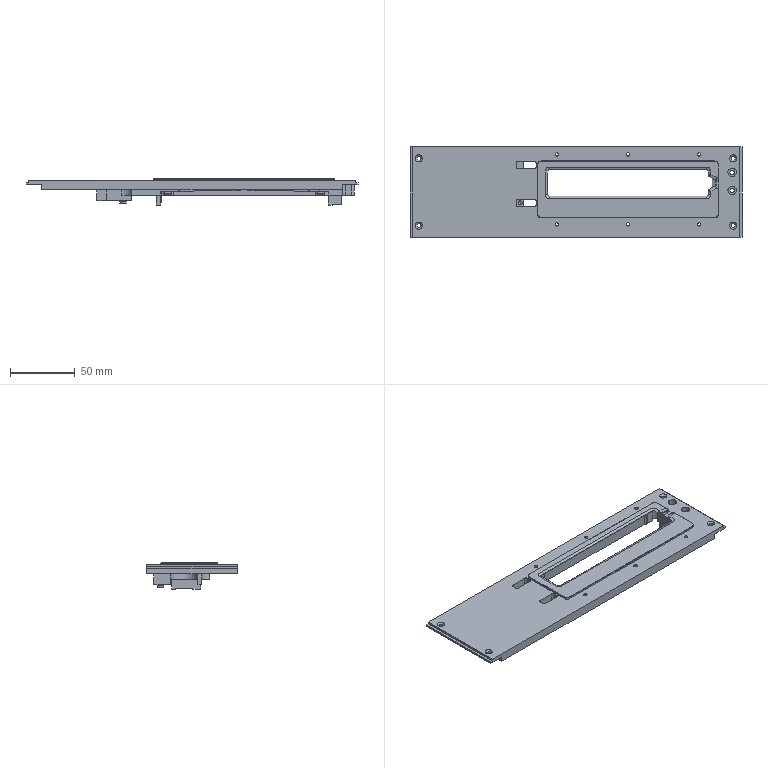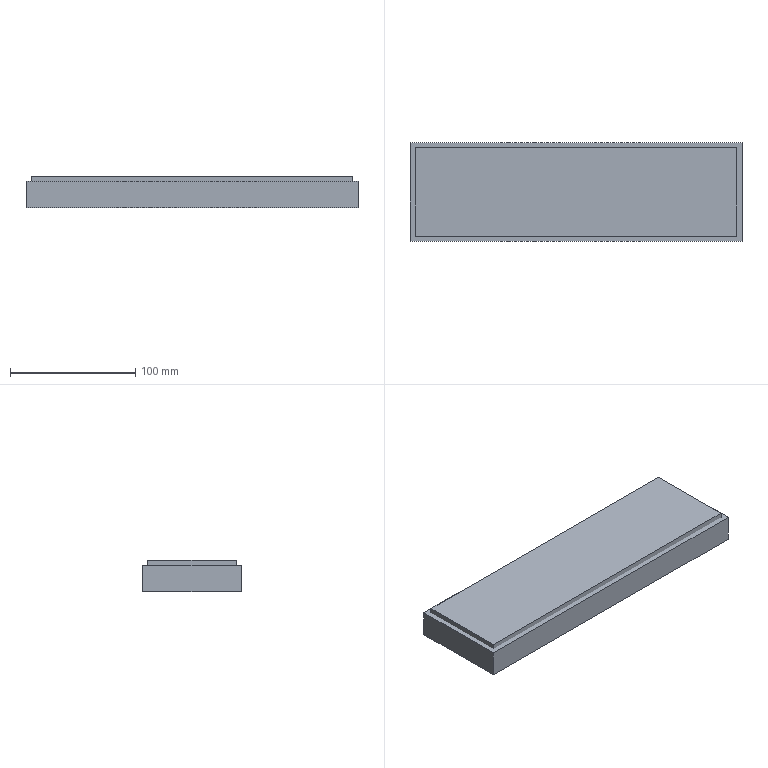CAM job | NX | 3-axis milling, drilling | part box 256.6 x 70.3 x 20.422 mm | stock box 264.6 x 78.3 x 25.422 mm
Tools:
number,name,description,diameter,corner_radius,flute_length,length,flutes
1,D63,Milling Tool-5 Parameters,63.0,0.0,50.0,75.0,2
10,D10,Milling Tool-5 Parameters,10.0,0.0,50.0,75.0,2
7,D6A45,Milling Tool-5 Parameters,6.0,0.0,3.0,3.0,2
13,3.2ZT,Drilling Tool,3.2,0.0,35.0,50.0,2
12,2.6ZT,Drilling Tool,2.6,0.0,35.0,50.0,2
14,3.4ZT,Drilling Tool,3.4,0.0,35.0,50.0,2
16,3.1ZT,Drilling Tool,3.1,0.0,35.0,50.0,2
6,D6,Milling Tool-5 Parameters,6.0,0.0,50.0,75.0,2
4,D4,Milling Tool-5 Parameters,4.0,0.0,50.0,75.0,2
3,D3,Milling Tool-5 Parameters,3.0,0.0,50.0,75.0,2
11,D10JING,Milling Tool-5 Parameters,10.0,0.0,50.0,75.0,2
2,D2,Milling Tool-5 Parameters,2.0,0.0,50.0,75.0,2
5,D2R0.5,Milling Tool-5 Parameters,2.0,0.5,50.0,75.0,2
15,D1.5,Milling Tool-5 Parameters,1.5,0.0,50.0,75.0,2
Operations:
program,operation,operation_type,tool,method,geometry_group,spindle_rpm,surface_speed,feed_per_tooth,feed_cut,feed_plunge,cut_length_mm,path_length_mm,cut_time_min,machine_time_min
PN_0001_BLANK,FLOOR_WALL,VolumeBased25DMillingOperation,D63,METHOD,A,6500.0,1286.0,0.0962,1250.0,100.0,1047.897,1101.897,0.8383,0.8437
PN_0001_BLANK,ADAPTIVE_MILLING,CavityMilling,D10,METHOD,A,9500.0,298.0,0.1579,3000.0,1000.0,22595.391,25583.451,8.469,8.767
PN_0001_BLANK,DRILLING,Operation,D6A45,METHOD,A,3500.0,43.0,0.0357,250.0,0.0,36.0,483.086,0.144,0.1887
PN_0001_BLANK,DRILLING_COPY_1,Operation,D6A45,METHOD,A,3500.0,43.0,0.0357,250.0,0.0,23.2,465.392,0.0928,0.137
PN_0001_BLANK,DRILLING_COPY_COPY,Operation,3.2ZT,METHOD,A,2500.0,19.0,0.024,120.0,0.0,34.346,487.683,0.2862,0.3315
PN_0001_BLANK,DRILLING_COPY_COPY_COPY,Operation,2.6ZT,METHOD,A,2500.0,19.0,0.024,120.0,0.0,74.263,498.74,0.6189,0.6613
PN_0001_BLANK,DRILLING_COPY_COPY_COPY_COPY,Operation,3.4ZT,METHOD,A,2500.0,19.0,0.024,120.0,0.0,33.643,147.404,0.2804,0.2917
PN_0001_BLANK,DRILLING_COPY_COPY_COPY_COPY_COPY,Operation,3.1ZT,METHOD,A,2500.0,19.0,0.024,120.0,0.0,12.601,88.002,0.105,0.1125
PN_0001_BLANK,ZLEVEL_PROFILE,ZLevelMilling,D6,METHOD,A,9500.0,179.0,0.0842,1600.0,100.0,235.589,850.61,0.1472,0.2087
PN_0001_BLANK,HOLE_MILLING,CylinderMilling,D3,METHOD,A,9500.0,89.0,0.0658,1250.0,100.0,736.533,890.125,0.5892,0.6046
PN_0001_BLANK,ZLEVEL_PROFILE_COPY,ZLevelMilling,D3,METHOD,A,9500.0,89.0,0.0632,1200.0,1000.0,1213.21,1283.978,1.015,1.022
PN_0001_BLANK,ZLEVEL_PROFILE_COPY_COPY,ZLevelMilling,D3,METHOD,A,9500.0,89.0,0.0632,1200.0,1000.0,1029.207,1097.302,0.8616,0.8684
PN_0001_BLANK,ZLEVEL_PROFILE_COPY_1,ZLevelMilling,D3,METHOD,A,9500.0,89.0,0.0632,1200.0,100.0,268.431,1301.32,0.2237,0.327
PN_0001_BLANK,ZLEVEL_PROFILE_COPY_COPY_1,ZLevelMilling,D3,METHOD,A,9500.0,89.0,0.0632,1200.0,1000.0,220.802,301.67,0.1879,0.196
PN_0001_BLANK,ZLEVEL_PROFILE_COPY_COPY_1_COPY,ZLevelMilling,D3,METHOD,A,9500.0,89.0,0.0632,1200.0,1000.0,342.85,422.245,0.2896,0.2976
PN_0001_BLANK,FLOOR_WALL_1_COPY,VolumeBased25DMillingOperation,D3,METHOD,A,9500.0,298.0,0.0658,1250.0,100.0,83.77,437.248,0.067,0.1024
PN_0001_BLANK,ZLEVEL_PROFILE_COPY_1_COPY,ZLevelMilling,D2,METHOD,A,9500.0,59.0,0.0526,1000.0,100.0,164.409,907.244,0.1644,0.2387
PN_0001_BLANK,ZLEVEL_PROFILE_1_COPY_1,ZLevelMilling,D2,METHOD,A,9500.0,59.0,0.0526,1000.0,100.0,287.955,351.033,0.288,0.2943
PN_0001_BLANK,ZLEVEL_PROFILE_COPY_COPY_1_1,ZLevelMilling,D2R0.5,METHOD,A,9500.0,59.0,0.1053,2000.0,1000.0,11195.633,11254.553,5.599,5.604
PN_0001_BLANK,FIXED_CONTOUR,SurfaceContour,D2R0.5,METHOD,A,9500.0,59.0,0.1053,2000.0,800.0,617.89,742.514,0.3323,0.3447
PN_0001_BLANK,ZLEVEL_PROFILE_1,ZLevelMilling,D10JING,METHOD,A,9500.0,298.0,0.0526,1000.0,100.0,694.216,792.059,0.6942,0.704
PN_0001_BLANK,ZLEVEL_PROFILE_1_COPY,ZLevelMilling,D10JING,METHOD,A,9500.0,298.0,0.0526,1000.0,100.0,179.973,572.806,0.18,0.2193
PN_0001_BLANK,FLOOR_WALL_1,VolumeBased25DMillingOperation,D10JING,METHOD,A,9500.0,298.0,0.0658,1250.0,100.0,2979.882,3291.972,2.384,2.415
PN_0001_BLANK,ZLEVEL_PROFILE_1_COPY_1_COPY_COPY,ZLevelMilling,D6A45,METHOD,A,9500.0,179.0,0.0526,1000.0,100.0,363.53,423.53,0.3635,0.3695
PN_0001_BLANK,ZLEVEL_PROFILE_1_COPY_1_COPY_COPY_COPY,ZLevelMilling,D6A45,METHOD,A,9500.0,179.0,0.0526,1000.0,100.0,816.983,2611.564,0.817,0.9964
2,FLOOR_WALL_COPY,VolumeBased25DMillingOperation,D63,METHOD,B,6500.0,1286.0,0.0962,1250.0,100.0,3481.485,3911.874,2.785,2.828
2,CAVITY_MILL,CavityMilling,D10,METHOD,B,9500.0,298.0,0.1579,3000.0,1000.0,62581.875,64537.882,21.301,21.497
2,CAVITY_MILL_COPY,CavityMilling,D6,METHOD,B,9500.0,179.0,0.0947,1800.0,1000.0,2401.348,4949.193,1.608,1.863
2,CAVITY_MILL_COPY_COPY,CavityMilling,D4,METHOD,B,9500.0,119.0,0.0737,1400.0,1000.0,3178.583,5927.303,2.506,2.781
2,ZLEVEL_PROFILE_1_COPY_COPY,ZLevelMilling,D4,METHOD,B,9500.0,298.0,0.0526,1000.0,100.0,657.009,752.791,0.657,0.6666
2,FLOOR_WALL_1_COPY_1,VolumeBased25DMillingOperation,D4,METHOD,B,9500.0,298.0,0.0658,1250.0,100.0,10849.161,16600.329,8.679,9.254
2,FLOOR_WALL_1_COPY_1_COPY,VolumeBased25DMillingOperation,D4,METHOD,B,9500.0,298.0,0.0658,1250.0,100.0,280.239,586.65,0.2242,0.2548
2,CAVITY_MILL_COPY_COPY_COPY,CavityMilling,D2,METHOD,B,9500.0,59.0,0.0526,1000.0,1000.0,2717.368,5468.507,2.717,2.993
2,DRILLING_COPY_COPY_COPY_COPY_1,Operation,D2,METHOD,B,2000.0,9.0,0.0125,50.0,0.0,17.7,125.518,0.354,0.3648
2,CAVITY_MILL_COPY_COPY_COPY_COPY,CavityMilling,D1.5,METHOD,B,9500.0,44.0,0.0447,850.0,1000.0,2219.123,3410.776,2.449,2.568
2,ZLEVEL_PROFILE_COPY_COPY_1_1_COPY,ZLevelMilling,D1.5,METHOD,B,9500.0,44.0,0.0789,1500.0,1000.0,2527.902,2803.528,1.686,1.714
2,ZLEVEL_PROFILE_COPY_COPY_1_1_COPY_1,ZLevelMilling,D2R0.5,METHOD,B,9500.0,59.0,0.1053,2000.0,1000.0,309.007,374.119,0.1563,0.1628
2,ZLEVEL_PROFILE_COPY_COPY_1_1_COPY_1_COPY,ZLevelMilling,D2R0.5,METHOD,B,9500.0,59.0,0.1053,2000.0,1000.0,367.827,637.55,0.1854,0.2124
2,ZLEVEL_PROFILE_COPY_COPY_1_1_COPY_1_COPY_COPY,ZLevelMilling,D2R0.5,METHOD,B,9500.0,59.0,0.1053,2000.0,1000.0,349.957,412.6,0.1757,0.182
2,ZLEVEL_PROFILE_COPY_COPY_1_1_COPY_1_COPY_COPY_COPY,ZLevelMilling,D2R0.5,METHOD,B,9500.0,59.0,0.1053,2000.0,1000.0,808.223,988.838,0.4069,0.4249
2,ZLEVEL_PROFILE_1_COPY_1_COPY_COPY_COPY_1,ZLevelMilling,D6A45,METHOD,B,9500.0,179.0,0.0526,1000.0,100.0,131.332,394.398,0.1313,0.1576
2,ZLEVEL_PROFILE_1_COPY_1_COPY_COPY_COPY_1_COPY,ZLevelMilling,D6A45,METHOD,B,9500.0,179.0,0.0526,1000.0,100.0,152.702,418.393,0.1527,0.1793
2,ZLEVEL_PROFILE_1_COPY_1_COPY_COPY_COPY_1_COPY_COPY,ZLevelMilling,D6A45,METHOD,B,9500.0,179.0,0.0526,1000.0,100.0,512.204,1943.135,0.5122,0.6553
2,ZLEVEL_PROFILE_1_COPY_1_COPY_COPY_COPY_1_COPY_COPY_COPY,ZLevelMilling,D6A45,METHOD,B,9500.0,179.0,0.0526,1000.0,100.0,719.416,1420.504,0.7194,0.7895
2,ZLEVEL_PROFILE_1_COPY_1_COPY_COPY_COPY_1_COPY_COPY_COPY_COPY,ZLevelMilling,D6A45,METHOD,B,9500.0,179.0,0.0526,1000.0,100.0,222.314,1762.768,0.2223,0.3764
2,CUTTER_COMP4,VolumeBased25DMillingOperation,D4,METHOD,B,9500.0,298.0,0.0658,1250.0,100.0,32.589,97.632,0.0261,0.0326